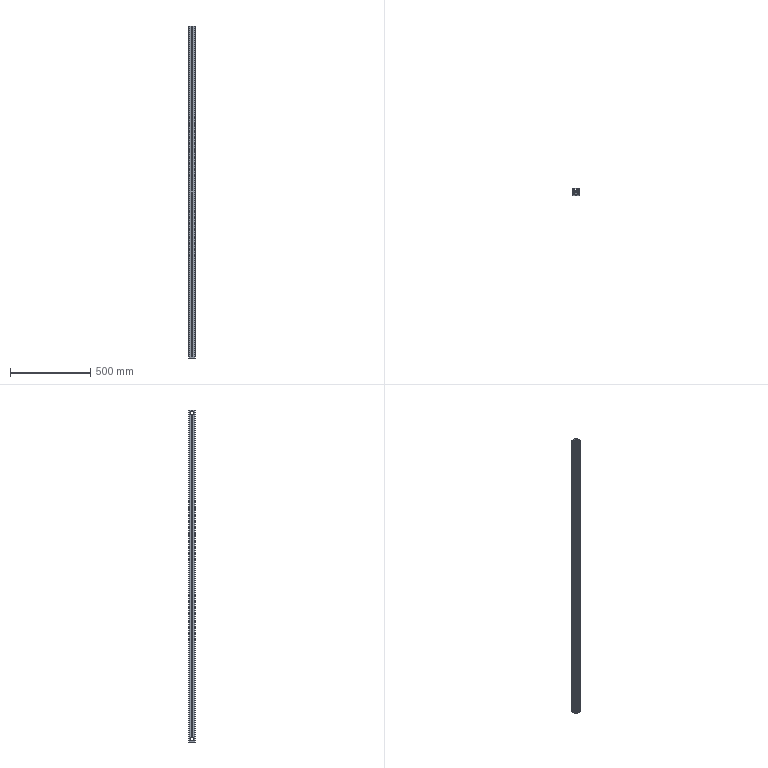Part | SolidWorks | features BaseBody 1, HoleWzd 1, MoveFace 1 | 1 solid | 242 faces | box 40 x 40 x 2066 mm | volume 1214839 mm3 | plane 187 | cylinder 55 | commonest cylinder face diameters 6.8 x15 2 x14 19 x12 1 x6 5 x4 9 x4